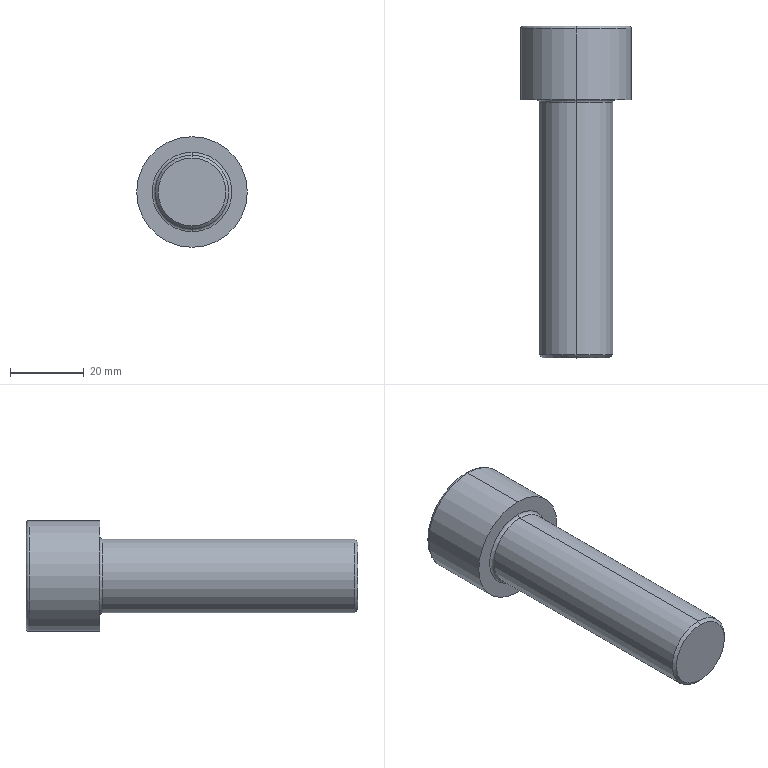Part | STEP file | 1 solid | 20 faces | box 30 x 90 x 30 mm | volume 33602 mm3 | plane 10 | torus 4 | cylinder 4 | cone 2 | commonest cylinder face diameters 20 x2 30 x2
STEP:
#1=CARTESIAN_POINT('',(0.,-70.,-9.2));
#2=VERTEX_POINT('',#1);
#3=CARTESIAN_POINT('',(0.,-70.,9.2));
#4=VERTEX_POINT('',#3);
#5=CARTESIAN_POINT('',(0.,-70.,0.));
#6=DIRECTION('',(0.,-1.,0.));
#7=DIRECTION('',(0.,0.,-1.));
#8=AXIS2_PLACEMENT_3D('',#5,#6,#7);
#9=CIRCLE('',#8,9.2);
#10=EDGE_CURVE('',#2,#4,#9,.T.);
#11=ORIENTED_EDGE('',*,*,#10,.F.);
#12=CARTESIAN_POINT('',(0.,-69.2,-10.));
#13=VERTEX_POINT('',#12);
#14=CARTESIAN_POINT('',(0.,-70.,-9.2));
#15=DIRECTION('',(0.,0.7071,-0.7071));
#16=VECTOR('',#15,1000.);
#17=LINE('',#14,#16);
#18=EDGE_CURVE('',#2,#13,#17,.T.);
#19=ORIENTED_EDGE('',*,*,#18,.T.);
#20=CARTESIAN_POINT('',(0.,-69.2,10.));
#21=VERTEX_POINT('',#20);
#22=CARTESIAN_POINT('',(0.,-69.2,0.));
#23=DIRECTION('',(0.,1.,0.));
#24=DIRECTION('',(0.,0.,-1.));
#25=AXIS2_PLACEMENT_3D('',#22,#23,#24);
#26=CIRCLE('',#25,10.);
#27=EDGE_CURVE('',#21,#13,#26,.T.);
#28=ORIENTED_EDGE('',*,*,#27,.F.);
#29=CARTESIAN_POINT('',(0.,-70.,9.2));
#30=DIRECTION('',(0.,0.7071,0.7071));
#31=VECTOR('',#30,1000.);
#32=LINE('',#29,#31);
#33=EDGE_CURVE('',#4,#21,#32,.T.);
#34=ORIENTED_EDGE('',*,*,#33,.F.);
#35=EDGE_LOOP('',(#11,#19,#28,#34));
#36=FACE_OUTER_BOUND('',#35,.T.);
#37=CARTESIAN_POINT('',(0.,-70.,0.));
#38=DIRECTION('',(0.,1.,0.));
#39=DIRECTION('',(0.,0.,1.));
#40=AXIS2_PLACEMENT_3D('',#37,#38,#39);
#41=CONICAL_SURFACE('',#40,9.2,0.7854);
#42=ADVANCED_FACE('',(#36),#41,.T.);
#43=CARTESIAN_POINT('',(0.,19.2,-15.));
#44=VERTEX_POINT('',#43);
#45=CARTESIAN_POINT('',(0.,19.2,15.));
#46=VERTEX_POINT('',#45);
#47=CARTESIAN_POINT('',(0.,19.2,0.));
#48=DIRECTION('',(0.,-1.,0.));
#49=DIRECTION('',(0.,0.,1.));
#50=AXIS2_PLACEMENT_3D('',#47,#48,#49);
#51=CIRCLE('',#50,15.);
#52=EDGE_CURVE('',#44,#46,#51,.T.);
#53=ORIENTED_EDGE('',*,*,#52,.F.);
#54=CARTESIAN_POINT('',(0.,20.,-14.2));
#55=VERTEX_POINT('',#54);
#56=CARTESIAN_POINT('',(0.,19.2,-14.2));
#57=DIRECTION('',(1.,0.,0.));
#58=DIRECTION('',(0.,0.,-1.));
#59=AXIS2_PLACEMENT_3D('',#56,#57,#58);
#60=CIRCLE('',#59,0.8);
#61=EDGE_CURVE('',#44,#55,#60,.T.);
#62=ORIENTED_EDGE('',*,*,#61,.T.);
#63=CARTESIAN_POINT('',(0.,20.,14.2));
#64=VERTEX_POINT('',#63);
#65=CARTESIAN_POINT('',(0.,20.,0.));
#66=DIRECTION('',(0.,1.,0.));
#67=DIRECTION('',(0.,0.,1.));
#68=AXIS2_PLACEMENT_3D('',#65,#66,#67);
#69=CIRCLE('',#68,14.2);
#70=EDGE_CURVE('',#64,#55,#69,.T.);
#71=ORIENTED_EDGE('',*,*,#70,.F.);
#72=CARTESIAN_POINT('',(0.,19.2,14.2));
#73=DIRECTION('',(-1.,0.,0.));
#74=DIRECTION('',(0.,0.,1.));
#75=AXIS2_PLACEMENT_3D('',#72,#73,#74);
#76=CIRCLE('',#75,0.8);
#77=EDGE_CURVE('',#46,#64,#76,.T.);
#78=ORIENTED_EDGE('',*,*,#77,.F.);
#79=EDGE_LOOP('',(#53,#62,#71,#78));
#80=FACE_OUTER_BOUND('',#79,.T.);
#81=CARTESIAN_POINT('',(0.,19.2,0.));
#82=DIRECTION('',(0.,1.,0.));
#83=DIRECTION('',(0.,0.,1.));
#84=AXIS2_PLACEMENT_3D('',#81,#82,#83);
#85=TOROIDAL_SURFACE('',#84,14.2,0.8);
#86=ADVANCED_FACE('',(#80),#85,.T.);
#87=CARTESIAN_POINT('',(0.,-0.8,10.));
#88=VERTEX_POINT('',#87);
#89=CARTESIAN_POINT('',(0.,-0.8,-10.));
#90=VERTEX_POINT('',#89);
#91=CARTESIAN_POINT('',(0.,-0.8,0.));
#92=DIRECTION('',(0.,-1.,0.));
#93=DIRECTION('',(0.,0.,-1.));
#94=AXIS2_PLACEMENT_3D('',#91,#92,#93);
#95=CIRCLE('',#94,10.);
#96=EDGE_CURVE('',#88,#90,#95,.T.);
#97=ORIENTED_EDGE('',*,*,#96,.F.);
#98=CARTESIAN_POINT('',(0.,0.,10.8));
#99=VERTEX_POINT('',#98);
#100=CARTESIAN_POINT('',(0.,-0.8,10.8));
#101=DIRECTION('',(1.,0.,0.));
#102=DIRECTION('',(0.,0.,-1.));
#103=AXIS2_PLACEMENT_3D('',#100,#101,#102);
#104=CIRCLE('',#103,0.8);
#105=EDGE_CURVE('',#88,#99,#104,.T.);
#106=ORIENTED_EDGE('',*,*,#105,.T.);
#107=CARTESIAN_POINT('',(0.,0.,-10.8));
#108=VERTEX_POINT('',#107);
#109=CARTESIAN_POINT('',(0.,0.,0.));
#110=DIRECTION('',(0.,1.,0.));
#111=DIRECTION('',(0.,0.,-1.));
#112=AXIS2_PLACEMENT_3D('',#109,#110,#111);
#113=CIRCLE('',#112,10.8);
#114=EDGE_CURVE('',#108,#99,#113,.T.);
#115=ORIENTED_EDGE('',*,*,#114,.F.);
#116=CARTESIAN_POINT('',(0.,-0.8,-10.8));
#117=DIRECTION('',(-1.,0.,0.));
#118=DIRECTION('',(0.,0.,1.));
#119=AXIS2_PLACEMENT_3D('',#116,#117,#118);
#120=CIRCLE('',#119,0.8);
#121=EDGE_CURVE('',#90,#108,#120,.T.);
#122=ORIENTED_EDGE('',*,*,#121,.F.);
#123=EDGE_LOOP('',(#97,#106,#115,#122));
#124=FACE_OUTER_BOUND('',#123,.T.);
#125=CARTESIAN_POINT('',(0.,-0.8,0.));
#126=DIRECTION('',(0.,-1.,0.));
#127=DIRECTION('',(0.,0.,-1.));
#128=AXIS2_PLACEMENT_3D('',#125,#126,#127);
#129=TOROIDAL_SURFACE('',#128,10.8,0.8);
#130=ADVANCED_FACE('',(#124),#129,.F.);
#131=CARTESIAN_POINT('',(0.,-0.8,0.));
#132=DIRECTION('',(0.,-1.,0.));
#133=DIRECTION('',(0.,0.,-1.));
#134=AXIS2_PLACEMENT_3D('',#131,#132,#133);
#135=CIRCLE('',#134,10.);
#136=EDGE_CURVE('',#90,#88,#135,.T.);
#137=ORIENTED_EDGE('',*,*,#136,.T.);
#138=CARTESIAN_POINT('',(0.,0.,10.));
#139=DIRECTION('',(0.,-1.,0.));
#140=VECTOR('',#139,1000.);
#141=LINE('',#138,#140);
#142=EDGE_CURVE('',#88,#21,#141,.T.);
#143=ORIENTED_EDGE('',*,*,#142,.T.);
#144=ORIENTED_EDGE('',*,*,#27,.T.);
#145=CARTESIAN_POINT('',(0.,0.,-10.));
#146=DIRECTION('',(0.,-1.,0.));
#147=VECTOR('',#146,1000.);
#148=LINE('',#145,#147);
#149=EDGE_CURVE('',#90,#13,#148,.T.);
#150=ORIENTED_EDGE('',*,*,#149,.F.);
#151=EDGE_LOOP('',(#137,#143,#144,#150));
#152=FACE_OUTER_BOUND('',#151,.T.);
#153=CARTESIAN_POINT('',(0.,0.,0.));
#154=DIRECTION('',(0.,-1.,0.));
#155=DIRECTION('',(0.,0.,-1.));
#156=AXIS2_PLACEMENT_3D('',#153,#154,#155);
#157=CYLINDRICAL_SURFACE('',#156,10.);
#158=ADVANCED_FACE('',(#152),#157,.T.);
#159=ORIENTED_EDGE('',*,*,#52,.T.);
#160=CARTESIAN_POINT('',(0.,0.,15.));
#161=VERTEX_POINT('',#160);
#162=CARTESIAN_POINT('',(0.,0.,15.));
#163=DIRECTION('',(0.,-1.,0.));
#164=VECTOR('',#163,1000.);
#165=LINE('',#162,#164);
#166=EDGE_CURVE('',#46,#161,#165,.T.);
#167=ORIENTED_EDGE('',*,*,#166,.T.);
#168=CARTESIAN_POINT('',(0.,0.,-15.));
#169=VERTEX_POINT('',#168);
#170=CARTESIAN_POINT('',(0.,0.,0.));
#171=DIRECTION('',(0.,-1.,0.));
#172=DIRECTION('',(0.,0.,-1.));
#173=AXIS2_PLACEMENT_3D('',#170,#171,#172);
#174=CIRCLE('',#173,15.);
#175=EDGE_CURVE('',#169,#161,#174,.T.);
#176=ORIENTED_EDGE('',*,*,#175,.F.);
#177=CARTESIAN_POINT('',(0.,0.,-15.));
#178=DIRECTION('',(0.,-1.,0.));
#179=VECTOR('',#178,1000.);
#180=LINE('',#177,#179);
#181=EDGE_CURVE('',#44,#169,#180,.T.);
#182=ORIENTED_EDGE('',*,*,#181,.F.);
#183=EDGE_LOOP('',(#159,#167,#176,#182));
#184=FACE_OUTER_BOUND('',#183,.T.);
#185=CARTESIAN_POINT('',(0.,0.,0.));
#186=DIRECTION('',(0.,-1.,0.));
#187=DIRECTION('',(0.,0.,-1.));
#188=AXIS2_PLACEMENT_3D('',#185,#186,#187);
#189=CYLINDRICAL_SURFACE('',#188,15.);
#190=ADVANCED_FACE('',(#184),#189,.T.);
#191=ORIENTED_EDGE('',*,*,#70,.T.);
#192=CARTESIAN_POINT('',(0.,20.,0.));
#193=DIRECTION('',(0.,1.,0.));
#194=DIRECTION('',(0.,0.,1.));
#195=AXIS2_PLACEMENT_3D('',#192,#193,#194);
#196=CIRCLE('',#195,14.2);
#197=EDGE_CURVE('',#55,#64,#196,.T.);
#198=ORIENTED_EDGE('',*,*,#197,.T.);
#199=EDGE_LOOP('',(#191,#198));
#200=FACE_OUTER_BOUND('',#199,.T.);
#201=CARTESIAN_POINT('',(0.,20.,-9.815));
#202=VERTEX_POINT('',#201);
#203=CARTESIAN_POINT('',(-8.5,20.,-4.907));
#204=VERTEX_POINT('',#203);
#205=CARTESIAN_POINT('',(0.,20.,-9.815));
#206=DIRECTION('',(-0.866,0.,0.5));
#207=VECTOR('',#206,1000.);
#208=LINE('',#205,#207);
#209=EDGE_CURVE('',#202,#204,#208,.T.);
#210=ORIENTED_EDGE('',*,*,#209,.F.);
#211=CARTESIAN_POINT('',(8.5,20.,-4.907));
#212=VERTEX_POINT('',#211);
#213=CARTESIAN_POINT('',(8.5,20.,-4.907));
#214=DIRECTION('',(-0.866,0.,-0.5));
#215=VECTOR('',#214,1000.);
#216=LINE('',#213,#215);
#217=EDGE_CURVE('',#212,#202,#216,.T.);
#218=ORIENTED_EDGE('',*,*,#217,.F.);
#219=CARTESIAN_POINT('',(8.5,20.,4.907));
#220=VERTEX_POINT('',#219);
#221=CARTESIAN_POINT('',(8.5,20.,4.907));
#222=DIRECTION('',(0.,0.,-1.));
#223=VECTOR('',#222,1000.);
#224=LINE('',#221,#223);
#225=EDGE_CURVE('',#220,#212,#224,.T.);
#226=ORIENTED_EDGE('',*,*,#225,.F.);
#227=CARTESIAN_POINT('',(0.,20.,9.815));
#228=VERTEX_POINT('',#227);
#229=CARTESIAN_POINT('',(0.,20.,9.815));
#230=DIRECTION('',(0.866,0.,-0.5));
#231=VECTOR('',#230,1000.);
#232=LINE('',#229,#231);
#233=EDGE_CURVE('',#228,#220,#232,.T.);
#234=ORIENTED_EDGE('',*,*,#233,.F.);
#235=CARTESIAN_POINT('',(-8.5,20.,4.907));
#236=VERTEX_POINT('',#235);
#237=CARTESIAN_POINT('',(-8.5,20.,4.907));
#238=DIRECTION('',(0.866,0.,0.5));
#239=VECTOR('',#238,1000.);
#240=LINE('',#237,#239);
#241=EDGE_CURVE('',#236,#228,#240,.T.);
#242=ORIENTED_EDGE('',*,*,#241,.F.);
#243=CARTESIAN_POINT('',(-8.5,20.,-4.907));
#244=DIRECTION('',(0.,0.,1.));
#245=VECTOR('',#244,1000.);
#246=LINE('',#243,#245);
#247=EDGE_CURVE('',#204,#236,#246,.T.);
#248=ORIENTED_EDGE('',*,*,#247,.F.);
#249=EDGE_LOOP('',(#210,#218,#226,#234,#242,#248));
#250=FACE_BOUND('',#249,.T.);
#251=CARTESIAN_POINT('',(0.,20.,0.));
#252=DIRECTION('',(0.,1.,0.));
#253=DIRECTION('',(0.,0.,1.));
#254=AXIS2_PLACEMENT_3D('',#251,#252,#253);
#255=PLANE('',#254);
#256=ADVANCED_FACE('',(#200,#250),#255,.T.);
#257=ORIENTED_EDGE('',*,*,#166,.F.);
#258=CARTESIAN_POINT('',(0.,19.2,0.));
#259=DIRECTION('',(0.,-1.,0.));
#260=DIRECTION('',(0.,0.,1.));
#261=AXIS2_PLACEMENT_3D('',#258,#259,#260);
#262=CIRCLE('',#261,15.);
#263=EDGE_CURVE('',#46,#44,#262,.T.);
#264=ORIENTED_EDGE('',*,*,#263,.T.);
#265=ORIENTED_EDGE('',*,*,#181,.T.);
#266=CARTESIAN_POINT('',(0.,0.,0.));
#267=DIRECTION('',(0.,-1.,0.));
#268=DIRECTION('',(0.,0.,-1.));
#269=AXIS2_PLACEMENT_3D('',#266,#267,#268);
#270=CIRCLE('',#269,15.);
#271=EDGE_CURVE('',#161,#169,#270,.T.);
#272=ORIENTED_EDGE('',*,*,#271,.F.);
#273=EDGE_LOOP('',(#257,#264,#265,#272));
#274=FACE_OUTER_BOUND('',#273,.T.);
#275=CARTESIAN_POINT('',(0.,0.,0.));
#276=DIRECTION('',(0.,-1.,0.));
#277=DIRECTION('',(0.,0.,-1.));
#278=AXIS2_PLACEMENT_3D('',#275,#276,#277);
#279=CYLINDRICAL_SURFACE('',#278,15.);
#280=ADVANCED_FACE('',(#274),#279,.T.);
#281=ORIENTED_EDGE('',*,*,#114,.T.);
#282=CARTESIAN_POINT('',(0.,0.,0.));
#283=DIRECTION('',(0.,1.,0.));
#284=DIRECTION('',(0.,0.,-1.));
#285=AXIS2_PLACEMENT_3D('',#282,#283,#284);
#286=CIRCLE('',#285,10.8);
#287=EDGE_CURVE('',#99,#108,#286,.T.);
#288=ORIENTED_EDGE('',*,*,#287,.T.);
#289=EDGE_LOOP('',(#281,#288));
#290=FACE_BOUND('',#289,.T.);
#291=ORIENTED_EDGE('',*,*,#175,.T.);
#292=ORIENTED_EDGE('',*,*,#271,.T.);
#293=EDGE_LOOP('',(#291,#292));
#294=FACE_OUTER_BOUND('',#293,.T.);
#295=CARTESIAN_POINT('',(15.,0.,0.));
#296=DIRECTION('',(0.,-1.,0.));
#297=DIRECTION('',(0.,0.,-1.));
#298=AXIS2_PLACEMENT_3D('',#295,#296,#297);
#299=PLANE('',#298);
#300=ADVANCED_FACE('',(#290,#294),#299,.T.);
#301=ORIENTED_EDGE('',*,*,#142,.F.);
#302=ORIENTED_EDGE('',*,*,#96,.T.);
#303=ORIENTED_EDGE('',*,*,#149,.T.);
#304=CARTESIAN_POINT('',(0.,-69.2,0.));
#305=DIRECTION('',(0.,1.,0.));
#306=DIRECTION('',(0.,0.,-1.));
#307=AXIS2_PLACEMENT_3D('',#304,#305,#306);
#308=CIRCLE('',#307,10.);
#309=EDGE_CURVE('',#13,#21,#308,.T.);
#310=ORIENTED_EDGE('',*,*,#309,.T.);
#311=EDGE_LOOP('',(#301,#302,#303,#310));
#312=FACE_OUTER_BOUND('',#311,.T.);
#313=CARTESIAN_POINT('',(0.,0.,0.));
#314=DIRECTION('',(0.,-1.,0.));
#315=DIRECTION('',(0.,0.,-1.));
#316=AXIS2_PLACEMENT_3D('',#313,#314,#315);
#317=CYLINDRICAL_SURFACE('',#316,10.);
#318=ADVANCED_FACE('',(#312),#317,.T.);
#319=CARTESIAN_POINT('',(0.,-70.,0.));
#320=DIRECTION('',(0.,-1.,0.));
#321=DIRECTION('',(0.,0.,-1.));
#322=AXIS2_PLACEMENT_3D('',#319,#320,#321);
#323=CIRCLE('',#322,9.2);
#324=EDGE_CURVE('',#4,#2,#323,.T.);
#325=ORIENTED_EDGE('',*,*,#324,.T.);
#326=ORIENTED_EDGE('',*,*,#10,.T.);
#327=EDGE_LOOP('',(#325,#326));
#328=FACE_OUTER_BOUND('',#327,.T.);
#329=CARTESIAN_POINT('',(10.,-70.,0.));
#330=DIRECTION('',(0.,-1.,0.));
#331=DIRECTION('',(0.,0.,-1.));
#332=AXIS2_PLACEMENT_3D('',#329,#330,#331);
#333=PLANE('',#332);
#334=ADVANCED_FACE('',(#328),#333,.T.);
#335=ORIENTED_EDGE('',*,*,#209,.T.);
#336=CARTESIAN_POINT('',(-8.5,10.,-4.907));
#337=VERTEX_POINT('',#336);
#338=CARTESIAN_POINT('',(-8.5,10.,-4.907));
#339=DIRECTION('',(0.,1.,0.));
#340=VECTOR('',#339,1000.);
#341=LINE('',#338,#340);
#342=EDGE_CURVE('',#337,#204,#341,.T.);
#343=ORIENTED_EDGE('',*,*,#342,.F.);
#344=CARTESIAN_POINT('',(0.,10.,-9.815));
#345=VERTEX_POINT('',#344);
#346=CARTESIAN_POINT('',(0.,10.,-9.815));
#347=DIRECTION('',(-0.866,0.,0.5));
#348=VECTOR('',#347,1000.);
#349=LINE('',#346,#348);
#350=EDGE_CURVE('',#345,#337,#349,.T.);
#351=ORIENTED_EDGE('',*,*,#350,.F.);
#352=CARTESIAN_POINT('',(0.,10.,-9.815));
#353=DIRECTION('',(0.,1.,0.));
#354=VECTOR('',#353,1000.);
#355=LINE('',#352,#354);
#356=EDGE_CURVE('',#345,#202,#355,.T.);
#357=ORIENTED_EDGE('',*,*,#356,.T.);
#358=EDGE_LOOP('',(#335,#343,#351,#357));
#359=FACE_OUTER_BOUND('',#358,.T.);
#360=CARTESIAN_POINT('',(0.,10.,-9.815));
#361=DIRECTION('',(-0.5,0.,-0.866));
#362=DIRECTION('',(-0.866,0.,0.5));
#363=AXIS2_PLACEMENT_3D('',#360,#361,#362);
#364=PLANE('',#363);
#365=ADVANCED_FACE('',(#359),#364,.F.);
#366=ORIENTED_EDGE('',*,*,#217,.T.);
#367=ORIENTED_EDGE('',*,*,#356,.F.);
#368=CARTESIAN_POINT('',(8.5,10.,-4.907));
#369=VERTEX_POINT('',#368);
#370=CARTESIAN_POINT('',(8.5,10.,-4.907));
#371=DIRECTION('',(-0.866,0.,-0.5));
#372=VECTOR('',#371,1000.);
#373=LINE('',#370,#372);
#374=EDGE_CURVE('',#369,#345,#373,.T.);
#375=ORIENTED_EDGE('',*,*,#374,.F.);
#376=CARTESIAN_POINT('',(8.5,10.,-4.907));
#377=DIRECTION('',(0.,1.,0.));
#378=VECTOR('',#377,1000.);
#379=LINE('',#376,#378);
#380=EDGE_CURVE('',#369,#212,#379,.T.);
#381=ORIENTED_EDGE('',*,*,#380,.T.);
#382=EDGE_LOOP('',(#366,#367,#375,#381));
#383=FACE_OUTER_BOUND('',#382,.T.);
#384=CARTESIAN_POINT('',(8.5,10.,-4.907));
#385=DIRECTION('',(0.5,0.,-0.866));
#386=DIRECTION('',(-0.866,0.,-0.5));
#387=AXIS2_PLACEMENT_3D('',#384,#385,#386);
#388=PLANE('',#387);
#389=ADVANCED_FACE('',(#383),#388,.F.);
#390=ORIENTED_EDGE('',*,*,#225,.T.);
#391=ORIENTED_EDGE('',*,*,#380,.F.);
#392=CARTESIAN_POINT('',(8.5,10.,4.907));
#393=VERTEX_POINT('',#392);
#394=CARTESIAN_POINT('',(8.5,10.,4.907));
#395=DIRECTION('',(0.,0.,-1.));
#396=VECTOR('',#395,1000.);
#397=LINE('',#394,#396);
#398=EDGE_CURVE('',#393,#369,#397,.T.);
#399=ORIENTED_EDGE('',*,*,#398,.F.);
#400=CARTESIAN_POINT('',(8.5,10.,4.907));
#401=DIRECTION('',(0.,1.,0.));
#402=VECTOR('',#401,1000.);
#403=LINE('',#400,#402);
#404=EDGE_CURVE('',#393,#220,#403,.T.);
#405=ORIENTED_EDGE('',*,*,#404,.T.);
#406=EDGE_LOOP('',(#390,#391,#399,#405));
#407=FACE_OUTER_BOUND('',#406,.T.);
#408=CARTESIAN_POINT('',(8.5,10.,4.907));
#409=DIRECTION('',(1.,0.,0.));
#410=DIRECTION('',(0.,0.,-1.));
#411=AXIS2_PLACEMENT_3D('',#408,#409,#410);
#412=PLANE('',#411);
#413=ADVANCED_FACE('',(#407),#412,.F.);
#414=ORIENTED_EDGE('',*,*,#233,.T.);
#415=ORIENTED_EDGE('',*,*,#404,.F.);
#416=CARTESIAN_POINT('',(0.,10.,9.815));
#417=VERTEX_POINT('',#416);
#418=CARTESIAN_POINT('',(0.,10.,9.815));
#419=DIRECTION('',(0.866,0.,-0.5));
#420=VECTOR('',#419,1000.);
#421=LINE('',#418,#420);
#422=EDGE_CURVE('',#417,#393,#421,.T.);
#423=ORIENTED_EDGE('',*,*,#422,.F.);
#424=CARTESIAN_POINT('',(0.,10.,9.815));
#425=DIRECTION('',(0.,1.,0.));
#426=VECTOR('',#425,1000.);
#427=LINE('',#424,#426);
#428=EDGE_CURVE('',#417,#228,#427,.T.);
#429=ORIENTED_EDGE('',*,*,#428,.T.);
#430=EDGE_LOOP('',(#414,#415,#423,#429));
#431=FACE_OUTER_BOUND('',#430,.T.);
#432=CARTESIAN_POINT('',(0.,10.,9.815));
#433=DIRECTION('',(0.5,0.,0.866));
#434=DIRECTION('',(0.866,0.,-0.5));
#435=AXIS2_PLACEMENT_3D('',#432,#433,#434);
#436=PLANE('',#435);
#437=ADVANCED_FACE('',(#431),#436,.F.);
#438=ORIENTED_EDGE('',*,*,#241,.T.);
#439=ORIENTED_EDGE('',*,*,#428,.F.);
#440=CARTESIAN_POINT('',(-8.5,10.,4.907));
#441=VERTEX_POINT('',#440);
#442=CARTESIAN_POINT('',(-8.5,10.,4.907));
#443=DIRECTION('',(0.866,0.,0.5));
#444=VECTOR('',#443,1000.);
#445=LINE('',#442,#444);
#446=EDGE_CURVE('',#441,#417,#445,.T.);
#447=ORIENTED_EDGE('',*,*,#446,.F.);
#448=CARTESIAN_POINT('',(-8.5,10.,4.907));
#449=DIRECTION('',(0.,1.,0.));
#450=VECTOR('',#449,1000.);
#451=LINE('',#448,#450);
#452=EDGE_CURVE('',#441,#236,#451,.T.);
#453=ORIENTED_EDGE('',*,*,#452,.T.);
#454=EDGE_LOOP('',(#438,#439,#447,#453));
#455=FACE_OUTER_BOUND('',#454,.T.);
#456=CARTESIAN_POINT('',(-8.5,10.,4.907));
#457=DIRECTION('',(-0.5,0.,0.866));
#458=DIRECTION('',(0.866,0.,0.5));
#459=AXIS2_PLACEMENT_3D('',#456,#457,#458);
#460=PLANE('',#459);
#461=ADVANCED_FACE('',(#455),#460,.F.);
#462=ORIENTED_EDGE('',*,*,#247,.T.);
#463=ORIENTED_EDGE('',*,*,#452,.F.);
#464=CARTESIAN_POINT('',(-8.5,10.,-4.907));
#465=DIRECTION('',(0.,0.,1.));
#466=VECTOR('',#465,1000.);
#467=LINE('',#464,#466);
#468=EDGE_CURVE('',#337,#441,#467,.T.);
#469=ORIENTED_EDGE('',*,*,#468,.F.);
#470=ORIENTED_EDGE('',*,*,#342,.T.);
#471=EDGE_LOOP('',(#462,#463,#469,#470));
#472=FACE_OUTER_BOUND('',#471,.T.);
#473=CARTESIAN_POINT('',(-8.5,10.,-4.907));
#474=DIRECTION('',(-1.,0.,0.));
#475=DIRECTION('',(0.,0.,1.));
#476=AXIS2_PLACEMENT_3D('',#473,#474,#475);
#477=PLANE('',#476);
#478=ADVANCED_FACE('',(#472),#477,.F.);
#479=ORIENTED_EDGE('',*,*,#350,.T.);
#480=ORIENTED_EDGE('',*,*,#468,.T.);
#481=ORIENTED_EDGE('',*,*,#446,.T.);
#482=ORIENTED_EDGE('',*,*,#422,.T.);
#483=ORIENTED_EDGE('',*,*,#398,.T.);
#484=ORIENTED_EDGE('',*,*,#374,.T.);
#485=EDGE_LOOP('',(#479,#480,#481,#482,#483,#484));
#486=FACE_OUTER_BOUND('',#485,.T.);
#487=CARTESIAN_POINT('',(0.,10.,0.));
#488=DIRECTION('',(0.,1.,0.));
#489=DIRECTION('',(0.,0.,1.));
#490=AXIS2_PLACEMENT_3D('',#487,#488,#489);
#491=PLANE('',#490);
#492=ADVANCED_FACE('',(#486),#491,.T.);
#493=ORIENTED_EDGE('',*,*,#105,.F.);
#494=ORIENTED_EDGE('',*,*,#136,.F.);
#495=ORIENTED_EDGE('',*,*,#121,.T.);
#496=ORIENTED_EDGE('',*,*,#287,.F.);
#497=EDGE_LOOP('',(#493,#494,#495,#496));
#498=FACE_OUTER_BOUND('',#497,.T.);
#499=CARTESIAN_POINT('',(0.,-0.8,0.));
#500=DIRECTION('',(0.,-1.,0.));
#501=DIRECTION('',(0.,0.,-1.));
#502=AXIS2_PLACEMENT_3D('',#499,#500,#501);
#503=TOROIDAL_SURFACE('',#502,10.8,0.8);
#504=ADVANCED_FACE('',(#498),#503,.F.);
#505=ORIENTED_EDGE('',*,*,#61,.F.);
#506=ORIENTED_EDGE('',*,*,#263,.F.);
#507=ORIENTED_EDGE('',*,*,#77,.T.);
#508=ORIENTED_EDGE('',*,*,#197,.F.);
#509=EDGE_LOOP('',(#505,#506,#507,#508));
#510=FACE_OUTER_BOUND('',#509,.T.);
#511=CARTESIAN_POINT('',(0.,19.2,0.));
#512=DIRECTION('',(0.,1.,0.));
#513=DIRECTION('',(0.,0.,1.));
#514=AXIS2_PLACEMENT_3D('',#511,#512,#513);
#515=TOROIDAL_SURFACE('',#514,14.2,0.8);
#516=ADVANCED_FACE('',(#510),#515,.T.);
#517=ORIENTED_EDGE('',*,*,#18,.F.);
#518=ORIENTED_EDGE('',*,*,#324,.F.);
#519=ORIENTED_EDGE('',*,*,#33,.T.);
#520=ORIENTED_EDGE('',*,*,#309,.F.);
#521=EDGE_LOOP('',(#517,#518,#519,#520));
#522=FACE_OUTER_BOUND('',#521,.T.);
#523=CARTESIAN_POINT('',(0.,-70.,0.));
#524=DIRECTION('',(0.,1.,0.));
#525=DIRECTION('',(0.,0.,1.));
#526=AXIS2_PLACEMENT_3D('',#523,#524,#525);
#527=CONICAL_SURFACE('',#526,9.2,0.7854);
#528=ADVANCED_FACE('',(#522),#527,.T.);
#529=CLOSED_SHELL('',(#42,#86,#130,#158,#190,#256,#280,#300,#318,#334,#365,#389,#413,#437,#461,#478,#492,#504,#516,#528));
#530=MANIFOLD_SOLID_BREP('',#529);
#531=CARTESIAN_POINT('',(0.,0.,0.));
#532=DIRECTION('',(0.,0.,1.));
#533=DIRECTION('',(1.,0.,0.));
#534=AXIS2_PLACEMENT_3D('',#531,#532,#533);
#535=(LENGTH_UNIT()NAMED_UNIT(*)SI_UNIT(.MILLI.,.METRE.));
#536=UNCERTAINTY_MEASURE_WITH_UNIT(LENGTH_MEASURE(0.00001),#535,'','');
#537=(NAMED_UNIT(*)PLANE_ANGLE_UNIT()SI_UNIT($,.RADIAN.));
#538=(NAMED_UNIT(*)SI_UNIT($,.STERADIAN.)SOLID_ANGLE_UNIT());
#539=(GEOMETRIC_REPRESENTATION_CONTEXT(3)GLOBAL_UNCERTAINTY_ASSIGNED_CONTEXT((#536))GLOBAL_UNIT_ASSIGNED_CONTEXT((#535,#537,#538))REPRESENTATION_CONTEXT('',''));
#540=ADVANCED_BREP_SHAPE_REPRESENTATION('',(#530,#534),#539);